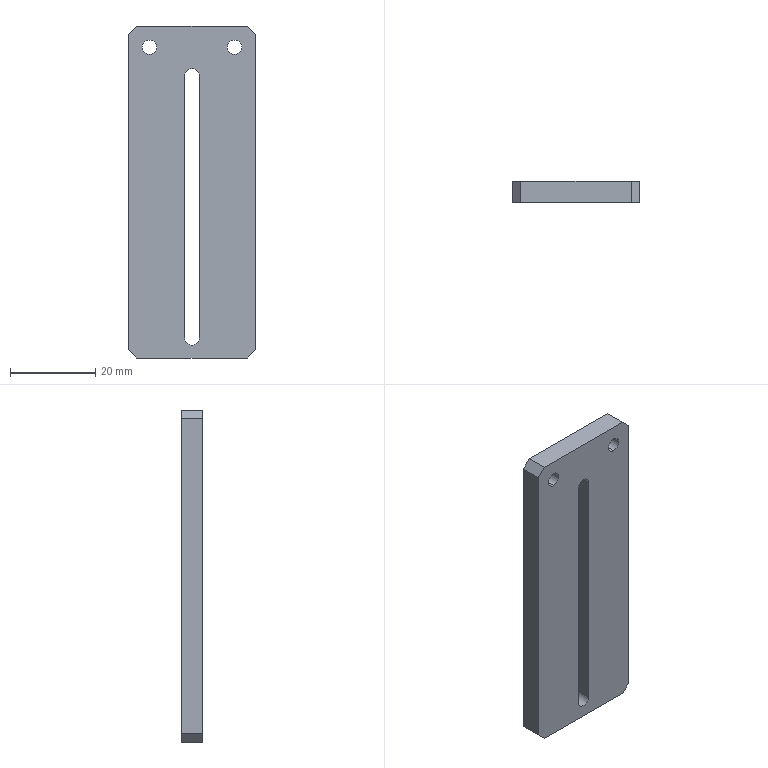Part | SolidWorks | features BaseBody 1 | 1 solid | 19 faces | box 30 x 5 x 78 mm | volume 10477 mm3 | plane 12 | cylinder 7 | commonest cylinder face diameters 3.4 x7
STEP:
#1=CARTESIAN_POINT('',(-10.,0.,32.3));
#2=VERTEX_POINT('',#1);
#3=CARTESIAN_POINT('',(-10.,0.,35.7));
#4=VERTEX_POINT('',#3);
#5=CARTESIAN_POINT('',(-10.,0.,34.));
#6=DIRECTION('',(0.,1.,0.));
#7=DIRECTION('',(0.,0.,1.));
#8=AXIS2_PLACEMENT_3D('',#5,#6,#7);
#9=CIRCLE('',#8,1.7);
#10=EDGE_CURVE('',#2,#4,#9,.T.);
#11=ORIENTED_EDGE('',*,*,#10,.F.);
#12=CARTESIAN_POINT('',(-10.,5.,32.3));
#13=VERTEX_POINT('',#12);
#14=CARTESIAN_POINT('',(-10.,5.,32.3));
#15=DIRECTION('',(0.,1.,0.));
#16=VECTOR('',#15,1000.);
#17=LINE('',#14,#16);
#18=EDGE_CURVE('',#2,#13,#17,.T.);
#19=ORIENTED_EDGE('',*,*,#18,.T.);
#20=CARTESIAN_POINT('',(-10.,5.,35.7));
#21=VERTEX_POINT('',#20);
#22=CARTESIAN_POINT('',(-10.,5.,34.));
#23=DIRECTION('',(0.,1.,0.));
#24=DIRECTION('',(0.,0.,1.));
#25=AXIS2_PLACEMENT_3D('',#22,#23,#24);
#26=CIRCLE('',#25,1.7);
#27=EDGE_CURVE('',#13,#21,#26,.T.);
#28=ORIENTED_EDGE('',*,*,#27,.T.);
#29=CARTESIAN_POINT('',(-10.,5.,35.7));
#30=DIRECTION('',(0.,1.,0.));
#31=VECTOR('',#30,1000.);
#32=LINE('',#29,#31);
#33=EDGE_CURVE('',#4,#21,#32,.T.);
#34=ORIENTED_EDGE('',*,*,#33,.F.);
#35=EDGE_LOOP('',(#11,#19,#28,#34));
#36=FACE_OUTER_BOUND('',#35,.T.);
#37=CARTESIAN_POINT('',(-10.,5.,34.));
#38=DIRECTION('',(0.,1.,0.));
#39=DIRECTION('',(0.,0.,1.));
#40=AXIS2_PLACEMENT_3D('',#37,#38,#39);
#41=CYLINDRICAL_SURFACE('',#40,1.7);
#42=ADVANCED_FACE('',(#36),#41,.F.);
#43=CARTESIAN_POINT('',(10.,0.,32.3));
#44=VERTEX_POINT('',#43);
#45=CARTESIAN_POINT('',(10.,0.,35.7));
#46=VERTEX_POINT('',#45);
#47=CARTESIAN_POINT('',(10.,0.,34.));
#48=DIRECTION('',(0.,1.,0.));
#49=DIRECTION('',(0.,0.,1.));
#50=AXIS2_PLACEMENT_3D('',#47,#48,#49);
#51=CIRCLE('',#50,1.7);
#52=EDGE_CURVE('',#44,#46,#51,.T.);
#53=ORIENTED_EDGE('',*,*,#52,.F.);
#54=CARTESIAN_POINT('',(10.,5.,32.3));
#55=VERTEX_POINT('',#54);
#56=CARTESIAN_POINT('',(10.,5.,32.3));
#57=DIRECTION('',(0.,1.,0.));
#58=VECTOR('',#57,1000.);
#59=LINE('',#56,#58);
#60=EDGE_CURVE('',#44,#55,#59,.T.);
#61=ORIENTED_EDGE('',*,*,#60,.T.);
#62=CARTESIAN_POINT('',(10.,5.,35.7));
#63=VERTEX_POINT('',#62);
#64=CARTESIAN_POINT('',(10.,5.,34.));
#65=DIRECTION('',(0.,1.,0.));
#66=DIRECTION('',(0.,0.,1.));
#67=AXIS2_PLACEMENT_3D('',#64,#65,#66);
#68=CIRCLE('',#67,1.7);
#69=EDGE_CURVE('',#55,#63,#68,.T.);
#70=ORIENTED_EDGE('',*,*,#69,.T.);
#71=CARTESIAN_POINT('',(10.,5.,35.7));
#72=DIRECTION('',(0.,1.,0.));
#73=VECTOR('',#72,1000.);
#74=LINE('',#71,#73);
#75=EDGE_CURVE('',#46,#63,#74,.T.);
#76=ORIENTED_EDGE('',*,*,#75,.F.);
#77=EDGE_LOOP('',(#53,#61,#70,#76));
#78=FACE_OUTER_BOUND('',#77,.T.);
#79=CARTESIAN_POINT('',(10.,5.,34.));
#80=DIRECTION('',(0.,1.,0.));
#81=DIRECTION('',(0.,0.,1.));
#82=AXIS2_PLACEMENT_3D('',#79,#80,#81);
#83=CYLINDRICAL_SURFACE('',#82,1.7);
#84=ADVANCED_FACE('',(#78),#83,.F.);
#85=CARTESIAN_POINT('',(0.,0.,29.));
#86=VERTEX_POINT('',#85);
#87=CARTESIAN_POINT('',(1.7,0.,27.3));
#88=VERTEX_POINT('',#87);
#89=CARTESIAN_POINT('',(0.,0.,27.3));
#90=DIRECTION('',(0.,1.,0.));
#91=DIRECTION('',(0.,0.,1.));
#92=AXIS2_PLACEMENT_3D('',#89,#90,#91);
#93=CIRCLE('',#92,1.7);
#94=EDGE_CURVE('',#86,#88,#93,.T.);
#95=ORIENTED_EDGE('',*,*,#94,.F.);
#96=CARTESIAN_POINT('',(0.,5.,29.));
#97=VERTEX_POINT('',#96);
#98=CARTESIAN_POINT('',(0.,5.,29.));
#99=DIRECTION('',(0.,1.,0.));
#100=VECTOR('',#99,1000.);
#101=LINE('',#98,#100);
#102=EDGE_CURVE('',#86,#97,#101,.T.);
#103=ORIENTED_EDGE('',*,*,#102,.T.);
#104=CARTESIAN_POINT('',(1.7,5.,27.3));
#105=VERTEX_POINT('',#104);
#106=CARTESIAN_POINT('',(0.,5.,27.3));
#107=DIRECTION('',(0.,1.,0.));
#108=DIRECTION('',(0.,0.,1.));
#109=AXIS2_PLACEMENT_3D('',#106,#107,#108);
#110=CIRCLE('',#109,1.7);
#111=EDGE_CURVE('',#97,#105,#110,.T.);
#112=ORIENTED_EDGE('',*,*,#111,.T.);
#113=CARTESIAN_POINT('',(1.7,0.,27.3));
#114=DIRECTION('',(0.,-1.,0.));
#115=VECTOR('',#114,1000.);
#116=LINE('',#113,#115);
#117=EDGE_CURVE('',#105,#88,#116,.T.);
#118=ORIENTED_EDGE('',*,*,#117,.T.);
#119=EDGE_LOOP('',(#95,#103,#112,#118));
#120=FACE_OUTER_BOUND('',#119,.T.);
#121=CARTESIAN_POINT('',(0.,5.,27.3));
#122=DIRECTION('',(0.,1.,0.));
#123=DIRECTION('',(0.,0.,1.));
#124=AXIS2_PLACEMENT_3D('',#121,#122,#123);
#125=CYLINDRICAL_SURFACE('',#124,1.7);
#126=ADVANCED_FACE('',(#120),#125,.F.);
#127=CARTESIAN_POINT('',(15.,5.,-37.));
#128=VERTEX_POINT('',#127);
#129=CARTESIAN_POINT('',(13.,5.,-39.));
#130=VERTEX_POINT('',#129);
#131=CARTESIAN_POINT('',(26.,5.,-26.));
#132=DIRECTION('',(-0.7071,0.,-0.7071));
#133=VECTOR('',#132,1000.);
#134=LINE('',#131,#133);
#135=EDGE_CURVE('',#128,#130,#134,.T.);
#136=ORIENTED_EDGE('',*,*,#135,.F.);
#137=CARTESIAN_POINT('',(15.,0.,-37.));
#138=VERTEX_POINT('',#137);
#139=CARTESIAN_POINT('',(15.,5.,-37.));
#140=DIRECTION('',(0.,1.,0.));
#141=VECTOR('',#140,1000.);
#142=LINE('',#139,#141);
#143=EDGE_CURVE('',#138,#128,#142,.T.);
#144=ORIENTED_EDGE('',*,*,#143,.F.);
#145=CARTESIAN_POINT('',(13.,0.,-39.));
#146=VERTEX_POINT('',#145);
#147=CARTESIAN_POINT('',(13.,0.,-39.));
#148=DIRECTION('',(0.7071,0.,0.7071));
#149=VECTOR('',#148,1000.);
#150=LINE('',#147,#149);
#151=EDGE_CURVE('',#146,#138,#150,.T.);
#152=ORIENTED_EDGE('',*,*,#151,.F.);
#153=CARTESIAN_POINT('',(13.,5.,-39.));
#154=DIRECTION('',(0.,-1.,0.));
#155=VECTOR('',#154,1000.);
#156=LINE('',#153,#155);
#157=EDGE_CURVE('',#130,#146,#156,.T.);
#158=ORIENTED_EDGE('',*,*,#157,.F.);
#159=EDGE_LOOP('',(#136,#144,#152,#158));
#160=FACE_OUTER_BOUND('',#159,.T.);
#161=CARTESIAN_POINT('',(13.,5.,-39.));
#162=DIRECTION('',(-0.7071,0.,0.7071));
#163=DIRECTION('',(0.,1.,0.));
#164=AXIS2_PLACEMENT_3D('',#161,#162,#163);
#165=PLANE('',#164);
#166=ADVANCED_FACE('',(#160),#165,.F.);
#167=CARTESIAN_POINT('',(-13.,5.,-39.));
#168=VERTEX_POINT('',#167);
#169=CARTESIAN_POINT('',(-15.,5.,-37.));
#170=VERTEX_POINT('',#169);
#171=CARTESIAN_POINT('',(-26.,5.,-26.));
#172=DIRECTION('',(-0.7071,0.,0.7071));
#173=VECTOR('',#172,1000.);
#174=LINE('',#171,#173);
#175=EDGE_CURVE('',#168,#170,#174,.T.);
#176=ORIENTED_EDGE('',*,*,#175,.F.);
#177=CARTESIAN_POINT('',(-13.,0.,-39.));
#178=VERTEX_POINT('',#177);
#179=CARTESIAN_POINT('',(-13.,5.,-39.));
#180=DIRECTION('',(0.,1.,0.));
#181=VECTOR('',#180,1000.);
#182=LINE('',#179,#181);
#183=EDGE_CURVE('',#178,#168,#182,.T.);
#184=ORIENTED_EDGE('',*,*,#183,.F.);
#185=CARTESIAN_POINT('',(-15.,0.,-37.));
#186=VERTEX_POINT('',#185);
#187=CARTESIAN_POINT('',(-15.,0.,-37.));
#188=DIRECTION('',(0.7071,0.,-0.7071));
#189=VECTOR('',#188,1000.);
#190=LINE('',#187,#189);
#191=EDGE_CURVE('',#186,#178,#190,.T.);
#192=ORIENTED_EDGE('',*,*,#191,.F.);
#193=CARTESIAN_POINT('',(-15.,5.,-37.));
#194=DIRECTION('',(0.,-1.,0.));
#195=VECTOR('',#194,1000.);
#196=LINE('',#193,#195);
#197=EDGE_CURVE('',#170,#186,#196,.T.);
#198=ORIENTED_EDGE('',*,*,#197,.F.);
#199=EDGE_LOOP('',(#176,#184,#192,#198));
#200=FACE_OUTER_BOUND('',#199,.T.);
#201=CARTESIAN_POINT('',(-15.,5.,-37.));
#202=DIRECTION('',(0.7071,0.,0.7071));
#203=DIRECTION('',(0.,-1.,0.));
#204=AXIS2_PLACEMENT_3D('',#201,#202,#203);
#205=PLANE('',#204);
#206=ADVANCED_FACE('',(#200),#205,.F.);
#207=CARTESIAN_POINT('',(13.,5.,39.));
#208=VERTEX_POINT('',#207);
#209=CARTESIAN_POINT('',(15.,5.,37.));
#210=VERTEX_POINT('',#209);
#211=CARTESIAN_POINT('',(26.,5.,26.));
#212=DIRECTION('',(0.7071,0.,-0.7071));
#213=VECTOR('',#212,1000.);
#214=LINE('',#211,#213);
#215=EDGE_CURVE('',#208,#210,#214,.T.);
#216=ORIENTED_EDGE('',*,*,#215,.F.);
#217=CARTESIAN_POINT('',(13.,0.,39.));
#218=VERTEX_POINT('',#217);
#219=CARTESIAN_POINT('',(13.,5.,39.));
#220=DIRECTION('',(0.,1.,0.));
#221=VECTOR('',#220,1000.);
#222=LINE('',#219,#221);
#223=EDGE_CURVE('',#218,#208,#222,.T.);
#224=ORIENTED_EDGE('',*,*,#223,.F.);
#225=CARTESIAN_POINT('',(15.,0.,37.));
#226=VERTEX_POINT('',#225);
#227=CARTESIAN_POINT('',(15.,0.,37.));
#228=DIRECTION('',(-0.7071,0.,0.7071));
#229=VECTOR('',#228,1000.);
#230=LINE('',#227,#229);
#231=EDGE_CURVE('',#226,#218,#230,.T.);
#232=ORIENTED_EDGE('',*,*,#231,.F.);
#233=CARTESIAN_POINT('',(15.,5.,37.));
#234=DIRECTION('',(0.,-1.,0.));
#235=VECTOR('',#234,1000.);
#236=LINE('',#233,#235);
#237=EDGE_CURVE('',#210,#226,#236,.T.);
#238=ORIENTED_EDGE('',*,*,#237,.F.);
#239=EDGE_LOOP('',(#216,#224,#232,#238));
#240=FACE_OUTER_BOUND('',#239,.T.);
#241=CARTESIAN_POINT('',(15.,5.,37.));
#242=DIRECTION('',(-0.7071,0.,-0.7071));
#243=DIRECTION('',(-0.7071,0.,0.7071));
#244=AXIS2_PLACEMENT_3D('',#241,#242,#243);
#245=PLANE('',#244);
#246=ADVANCED_FACE('',(#240),#245,.F.);
#247=CARTESIAN_POINT('',(-15.,5.,37.));
#248=VERTEX_POINT('',#247);
#249=CARTESIAN_POINT('',(-13.,5.,39.));
#250=VERTEX_POINT('',#249);
#251=CARTESIAN_POINT('',(-26.,5.,26.));
#252=DIRECTION('',(0.7071,0.,0.7071));
#253=VECTOR('',#252,1000.);
#254=LINE('',#251,#253);
#255=EDGE_CURVE('',#248,#250,#254,.T.);
#256=ORIENTED_EDGE('',*,*,#255,.F.);
#257=CARTESIAN_POINT('',(-15.,0.,37.));
#258=VERTEX_POINT('',#257);
#259=CARTESIAN_POINT('',(-15.,5.,37.));
#260=DIRECTION('',(0.,1.,0.));
#261=VECTOR('',#260,1000.);
#262=LINE('',#259,#261);
#263=EDGE_CURVE('',#258,#248,#262,.T.);
#264=ORIENTED_EDGE('',*,*,#263,.F.);
#265=CARTESIAN_POINT('',(-13.,0.,39.));
#266=VERTEX_POINT('',#265);
#267=CARTESIAN_POINT('',(-13.,0.,39.));
#268=DIRECTION('',(-0.7071,0.,-0.7071));
#269=VECTOR('',#268,1000.);
#270=LINE('',#267,#269);
#271=EDGE_CURVE('',#266,#258,#270,.T.);
#272=ORIENTED_EDGE('',*,*,#271,.F.);
#273=CARTESIAN_POINT('',(-13.,5.,39.));
#274=DIRECTION('',(0.,-1.,0.));
#275=VECTOR('',#274,1000.);
#276=LINE('',#273,#275);
#277=EDGE_CURVE('',#250,#266,#276,.T.);
#278=ORIENTED_EDGE('',*,*,#277,.F.);
#279=EDGE_LOOP('',(#256,#264,#272,#278));
#280=FACE_OUTER_BOUND('',#279,.T.);
#281=CARTESIAN_POINT('',(-13.,5.,39.));
#282=DIRECTION('',(0.7071,0.,-0.7071));
#283=DIRECTION('',(0.,-1.,0.));
#284=AXIS2_PLACEMENT_3D('',#281,#282,#283);
#285=PLANE('',#284);
#286=ADVANCED_FACE('',(#280),#285,.F.);
#287=CARTESIAN_POINT('',(-1.7,5.,27.3));
#288=VERTEX_POINT('',#287);
#289=CARTESIAN_POINT('',(-1.7,0.,27.3));
#290=VERTEX_POINT('',#289);
#291=CARTESIAN_POINT('',(-1.7,5.,27.3));
#292=DIRECTION('',(0.,-1.,0.));
#293=VECTOR('',#292,1000.);
#294=LINE('',#291,#293);
#295=EDGE_CURVE('',#288,#290,#294,.T.);
#296=ORIENTED_EDGE('',*,*,#295,.T.);
#297=CARTESIAN_POINT('',(-1.7,0.,-34.3));
#298=VERTEX_POINT('',#297);
#299=CARTESIAN_POINT('',(-1.7,0.,-34.3));
#300=DIRECTION('',(0.,0.,1.));
#301=VECTOR('',#300,1000.);
#302=LINE('',#299,#301);
#303=EDGE_CURVE('',#298,#290,#302,.T.);
#304=ORIENTED_EDGE('',*,*,#303,.F.);
#305=CARTESIAN_POINT('',(-1.7,5.,-34.3));
#306=VERTEX_POINT('',#305);
#307=CARTESIAN_POINT('',(-1.7,5.,-34.3));
#308=DIRECTION('',(0.,1.,0.));
#309=VECTOR('',#308,1000.);
#310=LINE('',#307,#309);
#311=EDGE_CURVE('',#298,#306,#310,.T.);
#312=ORIENTED_EDGE('',*,*,#311,.T.);
#313=CARTESIAN_POINT('',(-1.7,5.,-34.3));
#314=DIRECTION('',(0.,0.,1.));
#315=VECTOR('',#314,1000.);
#316=LINE('',#313,#315);
#317=EDGE_CURVE('',#306,#288,#316,.T.);
#318=ORIENTED_EDGE('',*,*,#317,.T.);
#319=EDGE_LOOP('',(#296,#304,#312,#318));
#320=FACE_OUTER_BOUND('',#319,.T.);
#321=CARTESIAN_POINT('',(-1.7,5.,-34.3));
#322=DIRECTION('',(-1.,0.,0.));
#323=DIRECTION('',(0.,1.,0.));
#324=AXIS2_PLACEMENT_3D('',#321,#322,#323);
#325=PLANE('',#324);
#326=ADVANCED_FACE('',(#320),#325,.F.);
#327=ORIENTED_EDGE('',*,*,#117,.F.);
#328=CARTESIAN_POINT('',(1.7,5.,-34.3));
#329=VERTEX_POINT('',#328);
#330=CARTESIAN_POINT('',(1.7,5.,-34.3));
#331=DIRECTION('',(0.,0.,1.));
#332=VECTOR('',#331,1000.);
#333=LINE('',#330,#332);
#334=EDGE_CURVE('',#329,#105,#333,.T.);
#335=ORIENTED_EDGE('',*,*,#334,.F.);
#336=CARTESIAN_POINT('',(1.7,0.,-34.3));
#337=VERTEX_POINT('',#336);
#338=CARTESIAN_POINT('',(1.7,0.,-34.3));
#339=DIRECTION('',(0.,-1.,0.));
#340=VECTOR('',#339,1000.);
#341=LINE('',#338,#340);
#342=EDGE_CURVE('',#329,#337,#341,.T.);
#343=ORIENTED_EDGE('',*,*,#342,.T.);
#344=CARTESIAN_POINT('',(1.7,0.,-34.3));
#345=DIRECTION('',(0.,0.,1.));
#346=VECTOR('',#345,1000.);
#347=LINE('',#344,#346);
#348=EDGE_CURVE('',#337,#88,#347,.T.);
#349=ORIENTED_EDGE('',*,*,#348,.T.);
#350=EDGE_LOOP('',(#327,#335,#343,#349));
#351=FACE_OUTER_BOUND('',#350,.T.);
#352=CARTESIAN_POINT('',(1.7,0.,-34.3));
#353=DIRECTION('',(-1.,0.,0.));
#354=DIRECTION('',(0.,1.,0.));
#355=AXIS2_PLACEMENT_3D('',#352,#353,#354);
#356=PLANE('',#355);
#357=ADVANCED_FACE('',(#351),#356,.T.);
#358=CARTESIAN_POINT('',(0.,0.,-34.3));
#359=DIRECTION('',(0.,1.,0.));
#360=DIRECTION('',(0.,0.,1.));
#361=AXIS2_PLACEMENT_3D('',#358,#359,#360);
#362=CIRCLE('',#361,1.7);
#363=EDGE_CURVE('',#337,#298,#362,.T.);
#364=ORIENTED_EDGE('',*,*,#363,.F.);
#365=ORIENTED_EDGE('',*,*,#342,.F.);
#366=CARTESIAN_POINT('',(0.,5.,-34.3));
#367=DIRECTION('',(0.,1.,0.));
#368=DIRECTION('',(0.,0.,1.));
#369=AXIS2_PLACEMENT_3D('',#366,#367,#368);
#370=CIRCLE('',#369,1.7);
#371=EDGE_CURVE('',#329,#306,#370,.T.);
#372=ORIENTED_EDGE('',*,*,#371,.T.);
#373=ORIENTED_EDGE('',*,*,#311,.F.);
#374=EDGE_LOOP('',(#364,#365,#372,#373));
#375=FACE_OUTER_BOUND('',#374,.T.);
#376=CARTESIAN_POINT('',(0.,5.,-34.3));
#377=DIRECTION('',(0.,1.,0.));
#378=DIRECTION('',(0.,0.,1.));
#379=AXIS2_PLACEMENT_3D('',#376,#377,#378);
#380=CYLINDRICAL_SURFACE('',#379,1.7);
#381=ADVANCED_FACE('',(#375),#380,.F.);
#382=ORIENTED_EDGE('',*,*,#303,.T.);
#383=CARTESIAN_POINT('',(0.,0.,27.3));
#384=DIRECTION('',(0.,1.,0.));
#385=DIRECTION('',(0.,0.,1.));
#386=AXIS2_PLACEMENT_3D('',#383,#384,#385);
#387=CIRCLE('',#386,1.7);
#388=EDGE_CURVE('',#290,#86,#387,.T.);
#389=ORIENTED_EDGE('',*,*,#388,.T.);
#390=ORIENTED_EDGE('',*,*,#94,.T.);
#391=ORIENTED_EDGE('',*,*,#348,.F.);
#392=ORIENTED_EDGE('',*,*,#363,.T.);
#393=EDGE_LOOP('',(#382,#389,#390,#391,#392));
#394=FACE_BOUND('',#393,.T.);
#395=CARTESIAN_POINT('',(10.,0.,34.));
#396=DIRECTION('',(0.,1.,0.));
#397=DIRECTION('',(0.,0.,1.));
#398=AXIS2_PLACEMENT_3D('',#395,#396,#397);
#399=CIRCLE('',#398,1.7);
#400=EDGE_CURVE('',#46,#44,#399,.T.);
#401=ORIENTED_EDGE('',*,*,#400,.T.);
#402=ORIENTED_EDGE('',*,*,#52,.T.);
#403=EDGE_LOOP('',(#401,#402));
#404=FACE_BOUND('',#403,.T.);
#405=CARTESIAN_POINT('',(-10.,0.,34.));
#406=DIRECTION('',(0.,1.,0.));
#407=DIRECTION('',(0.,0.,1.));
#408=AXIS2_PLACEMENT_3D('',#405,#406,#407);
#409=CIRCLE('',#408,1.7);
#410=EDGE_CURVE('',#4,#2,#409,.T.);
#411=ORIENTED_EDGE('',*,*,#410,.T.);
#412=ORIENTED_EDGE('',*,*,#10,.T.);
#413=EDGE_LOOP('',(#411,#412));
#414=FACE_BOUND('',#413,.T.);
#415=CARTESIAN_POINT('',(-15.,0.,39.));
#416=DIRECTION('',(1.,0.,0.));
#417=VECTOR('',#416,1000.);
#418=LINE('',#415,#417);
#419=EDGE_CURVE('',#266,#218,#418,.T.);
#420=ORIENTED_EDGE('',*,*,#419,.F.);
#421=ORIENTED_EDGE('',*,*,#271,.T.);
#422=CARTESIAN_POINT('',(-15.,0.,-39.));
#423=DIRECTION('',(0.,0.,1.));
#424=VECTOR('',#423,1000.);
#425=LINE('',#422,#424);
#426=EDGE_CURVE('',#186,#258,#425,.T.);
#427=ORIENTED_EDGE('',*,*,#426,.F.);
#428=ORIENTED_EDGE('',*,*,#191,.T.);
#429=CARTESIAN_POINT('',(-15.,0.,-39.));
#430=DIRECTION('',(-1.,0.,0.));
#431=VECTOR('',#430,1000.);
#432=LINE('',#429,#431);
#433=EDGE_CURVE('',#146,#178,#432,.T.);
#434=ORIENTED_EDGE('',*,*,#433,.F.);
#435=ORIENTED_EDGE('',*,*,#151,.T.);
#436=CARTESIAN_POINT('',(15.,0.,-39.));
#437=DIRECTION('',(0.,0.,-1.));
#438=VECTOR('',#437,1000.);
#439=LINE('',#436,#438);
#440=EDGE_CURVE('',#226,#138,#439,.T.);
#441=ORIENTED_EDGE('',*,*,#440,.F.);
#442=ORIENTED_EDGE('',*,*,#231,.T.);
#443=EDGE_LOOP('',(#420,#421,#427,#428,#434,#435,#441,#442));
#444=FACE_OUTER_BOUND('',#443,.T.);
#445=CARTESIAN_POINT('',(0.,0.,0.));
#446=DIRECTION('',(0.,1.,0.));
#447=DIRECTION('',(1.,0.,0.));
#448=AXIS2_PLACEMENT_3D('',#445,#446,#447);
#449=PLANE('',#448);
#450=ADVANCED_FACE('',(#394,#404,#414,#444),#449,.F.);
#451=CARTESIAN_POINT('',(-15.,5.,39.));
#452=DIRECTION('',(1.,0.,0.));
#453=VECTOR('',#452,1000.);
#454=LINE('',#451,#453);
#455=EDGE_CURVE('',#250,#208,#454,.T.);
#456=ORIENTED_EDGE('',*,*,#455,.F.);
#457=ORIENTED_EDGE('',*,*,#277,.T.);
#458=ORIENTED_EDGE('',*,*,#419,.T.);
#459=ORIENTED_EDGE('',*,*,#223,.T.);
#460=EDGE_LOOP('',(#456,#457,#458,#459));
#461=FACE_OUTER_BOUND('',#460,.T.);
#462=CARTESIAN_POINT('',(-15.,5.,39.));
#463=DIRECTION('',(0.,0.,-1.));
#464=DIRECTION('',(0.,-1.,0.));
#465=AXIS2_PLACEMENT_3D('',#462,#463,#464);
#466=PLANE('',#465);
#467=ADVANCED_FACE('',(#461),#466,.F.);
#468=ORIENTED_EDGE('',*,*,#426,.T.);
#469=ORIENTED_EDGE('',*,*,#263,.T.);
#470=CARTESIAN_POINT('',(-15.,5.,-39.));
#471=DIRECTION('',(0.,0.,1.));
#472=VECTOR('',#471,1000.);
#473=LINE('',#470,#472);
#474=EDGE_CURVE('',#170,#248,#473,.T.);
#475=ORIENTED_EDGE('',*,*,#474,.F.);
#476=ORIENTED_EDGE('',*,*,#197,.T.);
#477=EDGE_LOOP('',(#468,#469,#475,#476));
#478=FACE_OUTER_BOUND('',#477,.T.);
#479=CARTESIAN_POINT('',(-15.,5.,-39.));
#480=DIRECTION('',(1.,0.,0.));
#481=DIRECTION('',(0.,0.,-1.));
#482=AXIS2_PLACEMENT_3D('',#479,#480,#481);
#483=PLANE('',#482);
#484=ADVANCED_FACE('',(#478),#483,.F.);
#485=ORIENTED_EDGE('',*,*,#433,.T.);
#486=ORIENTED_EDGE('',*,*,#183,.T.);
#487=CARTESIAN_POINT('',(-15.,5.,-39.));
#488=DIRECTION('',(-1.,0.,0.));
#489=VECTOR('',#488,1000.);
#490=LINE('',#487,#489);
#491=EDGE_CURVE('',#130,#168,#490,.T.);
#492=ORIENTED_EDGE('',*,*,#491,.F.);
#493=ORIENTED_EDGE('',*,*,#157,.T.);
#494=EDGE_LOOP('',(#485,#486,#492,#493));
#495=FACE_OUTER_BOUND('',#494,.T.);
#496=CARTESIAN_POINT('',(-15.,5.,-39.));
#497=DIRECTION('',(0.,0.,1.));
#498=DIRECTION('',(1.,0.,0.));
#499=AXIS2_PLACEMENT_3D('',#496,#497,#498);
#500=PLANE('',#499);
#501=ADVANCED_FACE('',(#495),#500,.F.);
#502=CARTESIAN_POINT('',(15.,5.,-39.));
#503=DIRECTION('',(0.,0.,-1.));
#504=VECTOR('',#503,1000.);
#505=LINE('',#502,#504);
#506=EDGE_CURVE('',#210,#128,#505,.T.);
#507=ORIENTED_EDGE('',*,*,#506,.F.);
#508=ORIENTED_EDGE('',*,*,#237,.T.);
#509=ORIENTED_EDGE('',*,*,#440,.T.);
#510=ORIENTED_EDGE('',*,*,#143,.T.);
#511=EDGE_LOOP('',(#507,#508,#509,#510));
#512=FACE_OUTER_BOUND('',#511,.T.);
#513=CARTESIAN_POINT('',(15.,5.,-39.));
#514=DIRECTION('',(-1.,0.,0.));
#515=DIRECTION('',(0.,1.,0.));
#516=AXIS2_PLACEMENT_3D('',#513,#514,#515);
#517=PLANE('',#516);
#518=ADVANCED_FACE('',(#512),#517,.F.);
#519=ORIENTED_EDGE('',*,*,#371,.F.);
#520=ORIENTED_EDGE('',*,*,#334,.T.);
#521=ORIENTED_EDGE('',*,*,#111,.F.);
#522=CARTESIAN_POINT('',(0.,5.,27.3));
#523=DIRECTION('',(0.,1.,0.));
#524=DIRECTION('',(0.,0.,1.));
#525=AXIS2_PLACEMENT_3D('',#522,#523,#524);
#526=CIRCLE('',#525,1.7);
#527=EDGE_CURVE('',#288,#97,#526,.T.);
#528=ORIENTED_EDGE('',*,*,#527,.F.);
#529=ORIENTED_EDGE('',*,*,#317,.F.);
#530=EDGE_LOOP('',(#519,#520,#521,#528,#529));
#531=FACE_BOUND('',#530,.T.);
#532=CARTESIAN_POINT('',(10.,5.,34.));
#533=DIRECTION('',(0.,1.,0.));
#534=DIRECTION('',(0.,0.,1.));
#535=AXIS2_PLACEMENT_3D('',#532,#533,#534);
#536=CIRCLE('',#535,1.7);
#537=EDGE_CURVE('',#63,#55,#536,.T.);
#538=ORIENTED_EDGE('',*,*,#537,.F.);
#539=ORIENTED_EDGE('',*,*,#69,.F.);
#540=EDGE_LOOP('',(#538,#539));
#541=FACE_BOUND('',#540,.T.);
#542=CARTESIAN_POINT('',(-10.,5.,34.));
#543=DIRECTION('',(0.,1.,0.));
#544=DIRECTION('',(0.,0.,1.));
#545=AXIS2_PLACEMENT_3D('',#542,#543,#544);
#546=CIRCLE('',#545,1.7);
#547=EDGE_CURVE('',#21,#13,#546,.T.);
#548=ORIENTED_EDGE('',*,*,#547,.F.);
#549=ORIENTED_EDGE('',*,*,#27,.F.);
#550=EDGE_LOOP('',(#548,#549));
#551=FACE_BOUND('',#550,.T.);
#552=ORIENTED_EDGE('',*,*,#474,.T.);
#553=ORIENTED_EDGE('',*,*,#255,.T.);
#554=ORIENTED_EDGE('',*,*,#455,.T.);
#555=ORIENTED_EDGE('',*,*,#215,.T.);
#556=ORIENTED_EDGE('',*,*,#506,.T.);
#557=ORIENTED_EDGE('',*,*,#135,.T.);
#558=ORIENTED_EDGE('',*,*,#491,.T.);
#559=ORIENTED_EDGE('',*,*,#175,.T.);
#560=EDGE_LOOP('',(#552,#553,#554,#555,#556,#557,#558,#559));
#561=FACE_OUTER_BOUND('',#560,.T.);
#562=CARTESIAN_POINT('',(0.,5.,0.));
#563=DIRECTION('',(0.,1.,0.));
#564=DIRECTION('',(1.,0.,0.));
#565=AXIS2_PLACEMENT_3D('',#562,#563,#564);
#566=PLANE('',#565);
#567=ADVANCED_FACE('',(#531,#541,#551,#561),#566,.T.);
#568=ORIENTED_EDGE('',*,*,#102,.F.);
#569=ORIENTED_EDGE('',*,*,#388,.F.);
#570=ORIENTED_EDGE('',*,*,#295,.F.);
#571=ORIENTED_EDGE('',*,*,#527,.T.);
#572=EDGE_LOOP('',(#568,#569,#570,#571));
#573=FACE_OUTER_BOUND('',#572,.T.);
#574=CARTESIAN_POINT('',(0.,5.,27.3));
#575=DIRECTION('',(0.,1.,0.));
#576=DIRECTION('',(0.,0.,1.));
#577=AXIS2_PLACEMENT_3D('',#574,#575,#576);
#578=CYLINDRICAL_SURFACE('',#577,1.7);
#579=ADVANCED_FACE('',(#573),#578,.F.);
#580=ORIENTED_EDGE('',*,*,#60,.F.);
#581=ORIENTED_EDGE('',*,*,#400,.F.);
#582=ORIENTED_EDGE('',*,*,#75,.T.);
#583=ORIENTED_EDGE('',*,*,#537,.T.);
#584=EDGE_LOOP('',(#580,#581,#582,#583));
#585=FACE_OUTER_BOUND('',#584,.T.);
#586=CARTESIAN_POINT('',(10.,5.,34.));
#587=DIRECTION('',(0.,1.,0.));
#588=DIRECTION('',(0.,0.,1.));
#589=AXIS2_PLACEMENT_3D('',#586,#587,#588);
#590=CYLINDRICAL_SURFACE('',#589,1.7);
#591=ADVANCED_FACE('',(#585),#590,.F.);
#592=ORIENTED_EDGE('',*,*,#18,.F.);
#593=ORIENTED_EDGE('',*,*,#410,.F.);
#594=ORIENTED_EDGE('',*,*,#33,.T.);
#595=ORIENTED_EDGE('',*,*,#547,.T.);
#596=EDGE_LOOP('',(#592,#593,#594,#595));
#597=FACE_OUTER_BOUND('',#596,.T.);
#598=CARTESIAN_POINT('',(-10.,5.,34.));
#599=DIRECTION('',(0.,1.,0.));
#600=DIRECTION('',(0.,0.,1.));
#601=AXIS2_PLACEMENT_3D('',#598,#599,#600);
#602=CYLINDRICAL_SURFACE('',#601,1.7);
#603=ADVANCED_FACE('',(#597),#602,.F.);
#604=CLOSED_SHELL('',(#42,#84,#126,#166,#206,#246,#286,#326,#357,#381,#450,#467,#484,#501,#518,#567,#579,#591,#603));
#605=MANIFOLD_SOLID_BREP('',#604);
#606=CARTESIAN_POINT('',(0.,0.,0.));
#607=DIRECTION('',(0.,0.,1.));
#608=DIRECTION('',(1.,0.,0.));
#609=AXIS2_PLACEMENT_3D('',#606,#607,#608);
#610=(LENGTH_UNIT()NAMED_UNIT(*)SI_UNIT(.MILLI.,.METRE.));
#611=UNCERTAINTY_MEASURE_WITH_UNIT(LENGTH_MEASURE(0.00001),#610,'','');
#612=(NAMED_UNIT(*)PLANE_ANGLE_UNIT()SI_UNIT($,.RADIAN.));
#613=(NAMED_UNIT(*)SI_UNIT($,.STERADIAN.)SOLID_ANGLE_UNIT());
#614=(GEOMETRIC_REPRESENTATION_CONTEXT(3)GLOBAL_UNCERTAINTY_ASSIGNED_CONTEXT((#611))GLOBAL_UNIT_ASSIGNED_CONTEXT((#610,#612,#613))REPRESENTATION_CONTEXT('',''));
#615=ADVANCED_BREP_SHAPE_REPRESENTATION('',(#605,#609),#614);